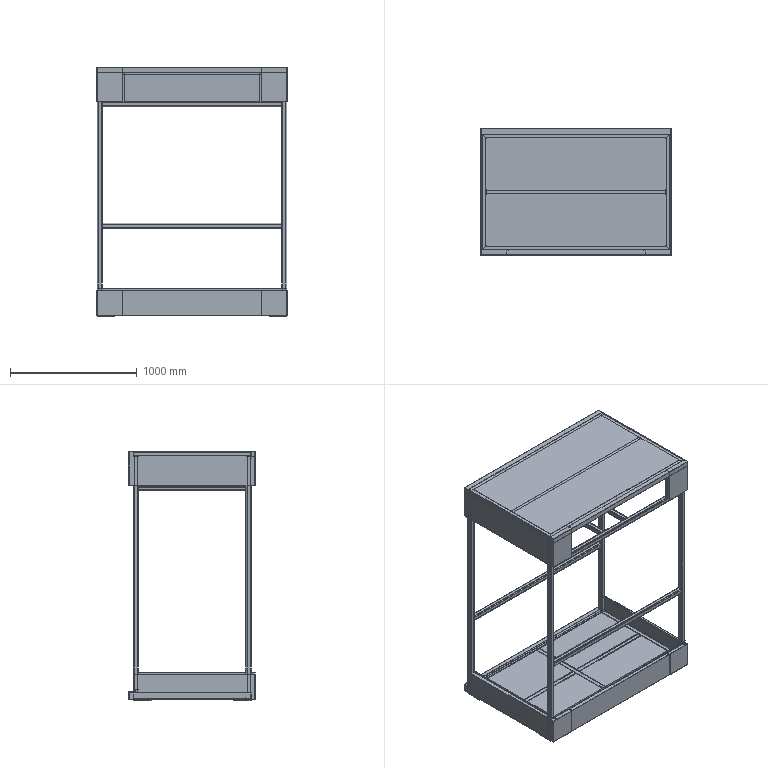Part | SolidWorks | features BaseBody 37 | 37 solids | 818 faces | box 1502 x 997.4 x 1969 mm | volume 37461315 mm3 | plane 558 | cylinder 260 | commonest cylinder face diameters 8 x72 16 x60 2 x36 6.4 x28 12.8 x28 4 x22